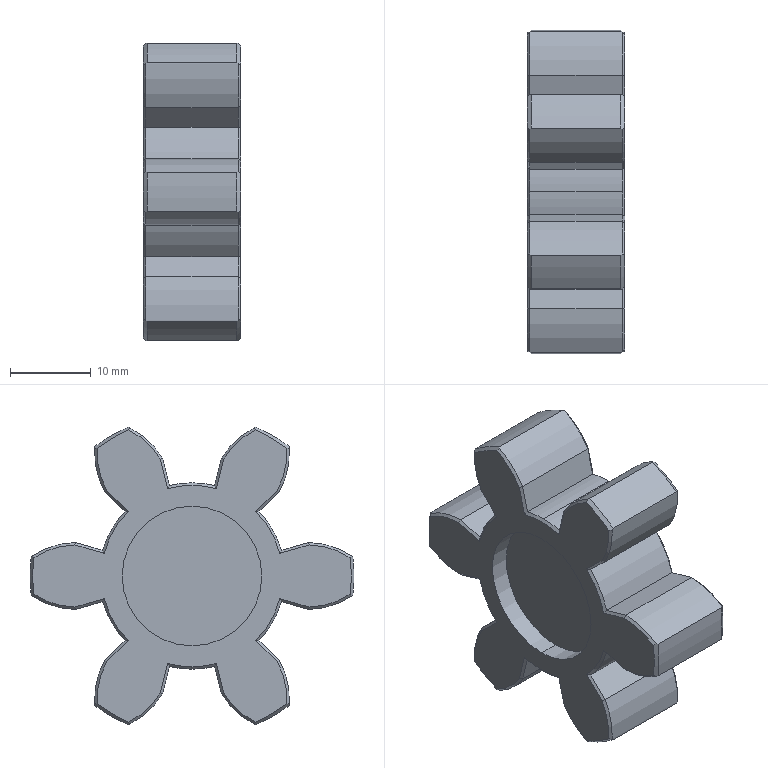Part | STEP file | D_BL_D40 | 1 solid | 119 faces | box 12 x 40 x 36.787 mm | volume 8300 mm3 | cone 50 | plane 40 | cylinder 29 | commonest cylinder face diameters 19.758 x12 23 x7 40 x6 17.25 x4